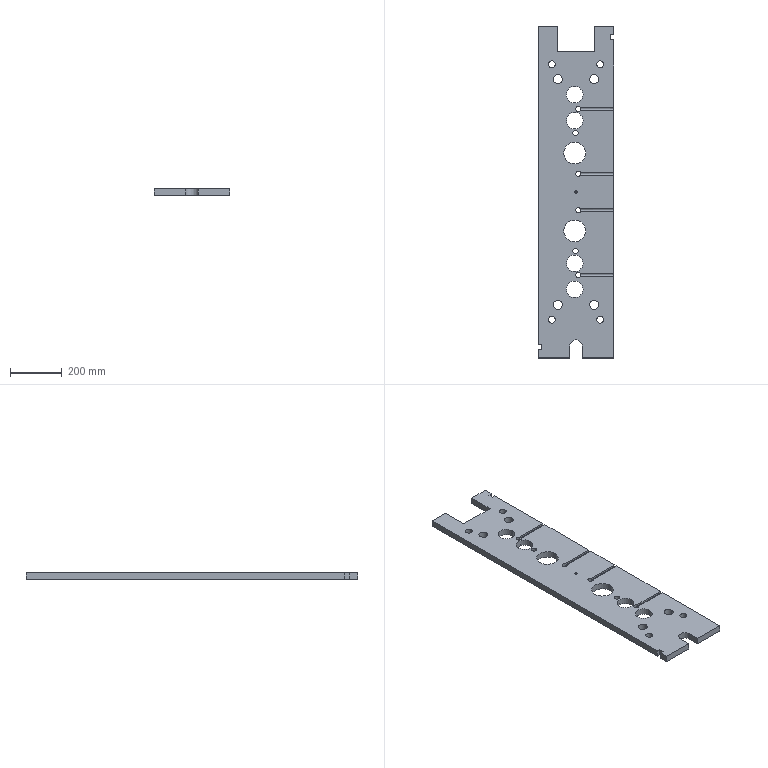Part | STEP file | 4-20.sldasm-Part-247 | 1 solid | 130 faces | box 290 x 1280 x 25 mm | volume 7957004 mm3 | cylinder 76 | plane 40 | torus 14 | commonest cylinder face diameters 26.4 x26 20.05 x12 32.75 x8 34.9 x8 64 x8 10.728 x4